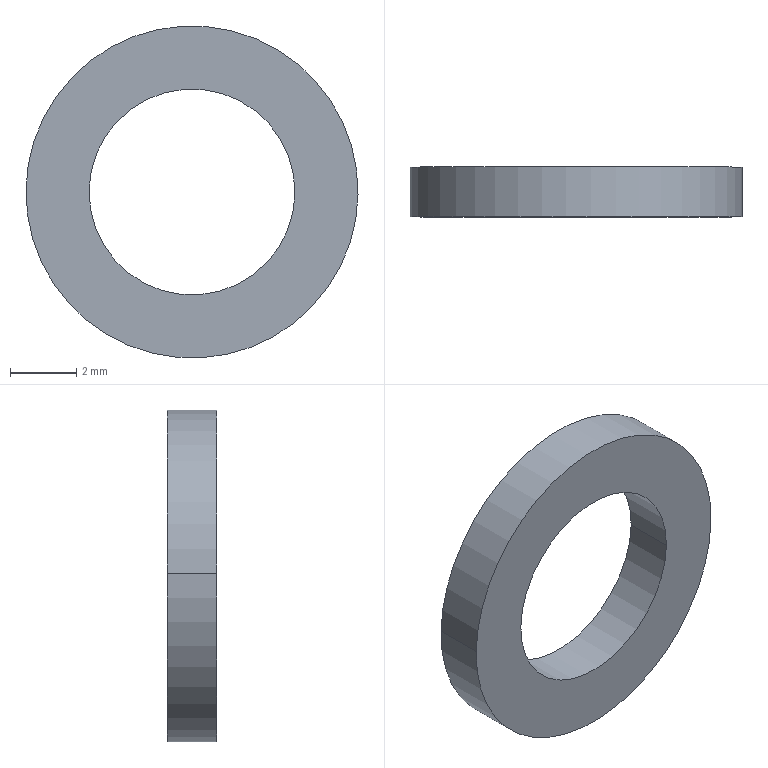Part | SolidWorks | features BaseBody 1 | 1 solid | 6 faces | box 10 x 1.5 x 10 mm | volume 72.524 mm3 | cylinder 4 | plane 2 | commonest cylinder face diameters 6.2 x2 10 x2
STEP:
#1=CARTESIAN_POINT('',(296.2,262.3,0.05112));
#2=VERTEX_POINT('',#1);
#3=CARTESIAN_POINT('',(302.4,262.3,-0.05112));
#4=VERTEX_POINT('',#3);
#5=CARTESIAN_POINT('',(299.3,262.3,0.));
#6=DIRECTION('',(0.,-1.,0.));
#7=DIRECTION('',(0.9999,0.,-0.01649));
#8=AXIS2_PLACEMENT_3D('',#5,#6,#7);
#9=CIRCLE('',#8,3.1);
#10=EDGE_CURVE('',#2,#4,#9,.T.);
#11=ORIENTED_EDGE('',*,*,#10,.T.);
#12=CARTESIAN_POINT('',(302.4,263.8,-0.05112));
#13=VERTEX_POINT('',#12);
#14=CARTESIAN_POINT('',(302.4,262.3,-0.05112));
#15=DIRECTION('',(0.,1.,0.));
#16=VECTOR('',#15,1000.);
#17=LINE('',#14,#16);
#18=EDGE_CURVE('',#4,#13,#17,.T.);
#19=ORIENTED_EDGE('',*,*,#18,.T.);
#20=CARTESIAN_POINT('',(296.2,263.8,0.05112));
#21=VERTEX_POINT('',#20);
#22=CARTESIAN_POINT('',(299.3,263.8,0.));
#23=DIRECTION('',(0.,-1.,0.));
#24=DIRECTION('',(0.9999,0.,-0.01649));
#25=AXIS2_PLACEMENT_3D('',#22,#23,#24);
#26=CIRCLE('',#25,3.1);
#27=EDGE_CURVE('',#21,#13,#26,.T.);
#28=ORIENTED_EDGE('',*,*,#27,.F.);
#29=CARTESIAN_POINT('',(296.2,262.3,0.05112));
#30=DIRECTION('',(0.,1.,0.));
#31=VECTOR('',#30,1000.);
#32=LINE('',#29,#31);
#33=EDGE_CURVE('',#2,#21,#32,.T.);
#34=ORIENTED_EDGE('',*,*,#33,.F.);
#35=EDGE_LOOP('',(#11,#19,#28,#34));
#36=FACE_OUTER_BOUND('',#35,.T.);
#37=CARTESIAN_POINT('',(299.3,262.3,0.));
#38=DIRECTION('',(0.,1.,0.));
#39=DIRECTION('',(-0.9999,0.,0.01649));
#40=AXIS2_PLACEMENT_3D('',#37,#38,#39);
#41=CYLINDRICAL_SURFACE('',#40,3.1);
#42=ADVANCED_FACE('',(#36),#41,.F.);
#43=CARTESIAN_POINT('',(304.299,262.3,-0.08245));
#44=VERTEX_POINT('',#43);
#45=CARTESIAN_POINT('',(294.301,262.3,0.08245));
#46=VERTEX_POINT('',#45);
#47=CARTESIAN_POINT('',(299.3,262.3,0.));
#48=DIRECTION('',(0.,-1.,0.));
#49=DIRECTION('',(0.9999,0.,-0.01649));
#50=AXIS2_PLACEMENT_3D('',#47,#48,#49);
#51=CIRCLE('',#50,5.);
#52=EDGE_CURVE('',#44,#46,#51,.T.);
#53=ORIENTED_EDGE('',*,*,#52,.F.);
#54=CARTESIAN_POINT('',(304.299,263.8,-0.08245));
#55=VERTEX_POINT('',#54);
#56=CARTESIAN_POINT('',(304.299,262.3,-0.08245));
#57=DIRECTION('',(0.,1.,0.));
#58=VECTOR('',#57,1000.);
#59=LINE('',#56,#58);
#60=EDGE_CURVE('',#44,#55,#59,.T.);
#61=ORIENTED_EDGE('',*,*,#60,.T.);
#62=CARTESIAN_POINT('',(294.301,263.8,0.08245));
#63=VERTEX_POINT('',#62);
#64=CARTESIAN_POINT('',(299.3,263.8,0.));
#65=DIRECTION('',(0.,-1.,0.));
#66=DIRECTION('',(0.9999,0.,-0.01649));
#67=AXIS2_PLACEMENT_3D('',#64,#65,#66);
#68=CIRCLE('',#67,5.);
#69=EDGE_CURVE('',#55,#63,#68,.T.);
#70=ORIENTED_EDGE('',*,*,#69,.T.);
#71=CARTESIAN_POINT('',(294.301,262.3,0.08245));
#72=DIRECTION('',(0.,1.,0.));
#73=VECTOR('',#72,1000.);
#74=LINE('',#71,#73);
#75=EDGE_CURVE('',#46,#63,#74,.T.);
#76=ORIENTED_EDGE('',*,*,#75,.F.);
#77=EDGE_LOOP('',(#53,#61,#70,#76));
#78=FACE_OUTER_BOUND('',#77,.T.);
#79=CARTESIAN_POINT('',(299.3,262.3,0.));
#80=DIRECTION('',(0.,1.,0.));
#81=DIRECTION('',(-0.9999,0.,0.01649));
#82=AXIS2_PLACEMENT_3D('',#79,#80,#81);
#83=CYLINDRICAL_SURFACE('',#82,5.);
#84=ADVANCED_FACE('',(#78),#83,.T.);
#85=CARTESIAN_POINT('',(299.3,262.3,0.));
#86=DIRECTION('',(0.,-1.,0.));
#87=DIRECTION('',(0.9999,0.,-0.01649));
#88=AXIS2_PLACEMENT_3D('',#85,#86,#87);
#89=CIRCLE('',#88,5.);
#90=EDGE_CURVE('',#46,#44,#89,.T.);
#91=ORIENTED_EDGE('',*,*,#90,.T.);
#92=ORIENTED_EDGE('',*,*,#52,.T.);
#93=EDGE_LOOP('',(#91,#92));
#94=FACE_OUTER_BOUND('',#93,.T.);
#95=ORIENTED_EDGE('',*,*,#10,.F.);
#96=CARTESIAN_POINT('',(299.3,262.3,0.));
#97=DIRECTION('',(0.,-1.,0.));
#98=DIRECTION('',(0.9999,0.,-0.01649));
#99=AXIS2_PLACEMENT_3D('',#96,#97,#98);
#100=CIRCLE('',#99,3.1);
#101=EDGE_CURVE('',#4,#2,#100,.T.);
#102=ORIENTED_EDGE('',*,*,#101,.F.);
#103=EDGE_LOOP('',(#95,#102));
#104=FACE_BOUND('',#103,.T.);
#105=CARTESIAN_POINT('',(299.3,262.3,0.));
#106=DIRECTION('',(0.,-1.,0.));
#107=DIRECTION('',(0.9999,0.,-0.01649));
#108=AXIS2_PLACEMENT_3D('',#105,#106,#107);
#109=PLANE('',#108);
#110=ADVANCED_FACE('',(#94,#104),#109,.T.);
#111=CARTESIAN_POINT('',(299.3,263.8,0.));
#112=DIRECTION('',(0.,-1.,0.));
#113=DIRECTION('',(0.9999,0.,-0.01649));
#114=AXIS2_PLACEMENT_3D('',#111,#112,#113);
#115=CIRCLE('',#114,5.);
#116=EDGE_CURVE('',#63,#55,#115,.T.);
#117=ORIENTED_EDGE('',*,*,#116,.F.);
#118=ORIENTED_EDGE('',*,*,#69,.F.);
#119=EDGE_LOOP('',(#117,#118));
#120=FACE_OUTER_BOUND('',#119,.T.);
#121=ORIENTED_EDGE('',*,*,#27,.T.);
#122=CARTESIAN_POINT('',(299.3,263.8,0.));
#123=DIRECTION('',(0.,-1.,0.));
#124=DIRECTION('',(0.9999,0.,-0.01649));
#125=AXIS2_PLACEMENT_3D('',#122,#123,#124);
#126=CIRCLE('',#125,3.1);
#127=EDGE_CURVE('',#13,#21,#126,.T.);
#128=ORIENTED_EDGE('',*,*,#127,.T.);
#129=EDGE_LOOP('',(#121,#128));
#130=FACE_BOUND('',#129,.T.);
#131=CARTESIAN_POINT('',(299.3,263.8,0.));
#132=DIRECTION('',(0.,-1.,0.));
#133=DIRECTION('',(0.9999,0.,-0.01649));
#134=AXIS2_PLACEMENT_3D('',#131,#132,#133);
#135=PLANE('',#134);
#136=ADVANCED_FACE('',(#120,#130),#135,.F.);
#137=ORIENTED_EDGE('',*,*,#60,.F.);
#138=ORIENTED_EDGE('',*,*,#90,.F.);
#139=ORIENTED_EDGE('',*,*,#75,.T.);
#140=ORIENTED_EDGE('',*,*,#116,.T.);
#141=EDGE_LOOP('',(#137,#138,#139,#140));
#142=FACE_OUTER_BOUND('',#141,.T.);
#143=CARTESIAN_POINT('',(299.3,262.3,0.));
#144=DIRECTION('',(0.,1.,0.));
#145=DIRECTION('',(-0.9999,0.,0.01649));
#146=AXIS2_PLACEMENT_3D('',#143,#144,#145);
#147=CYLINDRICAL_SURFACE('',#146,5.);
#148=ADVANCED_FACE('',(#142),#147,.T.);
#149=ORIENTED_EDGE('',*,*,#18,.F.);
#150=ORIENTED_EDGE('',*,*,#101,.T.);
#151=ORIENTED_EDGE('',*,*,#33,.T.);
#152=ORIENTED_EDGE('',*,*,#127,.F.);
#153=EDGE_LOOP('',(#149,#150,#151,#152));
#154=FACE_OUTER_BOUND('',#153,.T.);
#155=CARTESIAN_POINT('',(299.3,262.3,0.));
#156=DIRECTION('',(0.,1.,0.));
#157=DIRECTION('',(-0.9999,0.,0.01649));
#158=AXIS2_PLACEMENT_3D('',#155,#156,#157);
#159=CYLINDRICAL_SURFACE('',#158,3.1);
#160=ADVANCED_FACE('',(#154),#159,.F.);
#161=CLOSED_SHELL('',(#42,#84,#110,#136,#148,#160));
#162=MANIFOLD_SOLID_BREP('',#161);
#163=CARTESIAN_POINT('',(0.,0.,0.));
#164=DIRECTION('',(0.,0.,1.));
#165=DIRECTION('',(1.,0.,0.));
#166=AXIS2_PLACEMENT_3D('',#163,#164,#165);
#167=(LENGTH_UNIT()NAMED_UNIT(*)SI_UNIT(.MILLI.,.METRE.));
#168=UNCERTAINTY_MEASURE_WITH_UNIT(LENGTH_MEASURE(0.00001),#167,'','');
#169=(NAMED_UNIT(*)PLANE_ANGLE_UNIT()SI_UNIT($,.RADIAN.));
#170=(NAMED_UNIT(*)SI_UNIT($,.STERADIAN.)SOLID_ANGLE_UNIT());
#171=(GEOMETRIC_REPRESENTATION_CONTEXT(3)GLOBAL_UNCERTAINTY_ASSIGNED_CONTEXT((#168))GLOBAL_UNIT_ASSIGNED_CONTEXT((#167,#169,#170))REPRESENTATION_CONTEXT('',''));
#172=ADVANCED_BREP_SHAPE_REPRESENTATION('',(#162,#166),#171);